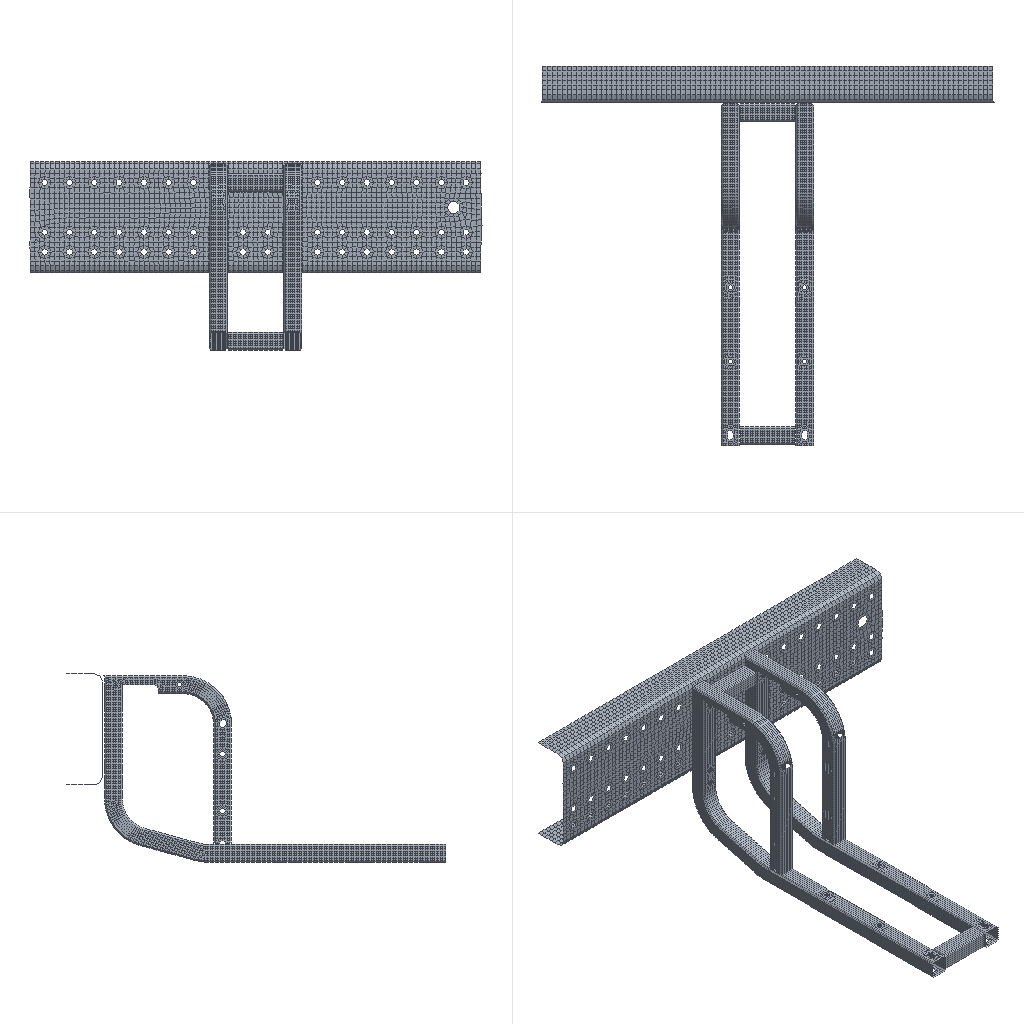Simulation study | nastran
Set-up summary:
category,name,step,type,value,unit,region
solver,nx_nastran
units,not stated in the deck,,not stated
analysis,deck,,static,static
analysis,solution,,SOL,101
load_step,SUBCASE 1,1,SUBCASE,SPC=6 LOAD=1
load_step,SUBCASE 2,2,SUBCASE,SPC=6 LOAD=2
load_step,SUBCASE 3,3,SUBCASE,SPC=6 LOAD=3
load_step,SUBCASE 4,4,SUBCASE,SPC=6 LOAD=4
load_step,requested,,,4
mesh,nodes,,,21323
mesh,elements,,,20706
element_type,CONM2,,mass,1
element_type,CQUAD4,,shell,20543
element_type,CTRIA3,,shell,162
load,load commands in deck,,count,4
bc,support commands in deck,,count,72
check,setup vs results,,match,"every grid point's frame and coordinates and every element id; grid points of CQUAD4, CTRIA3 elements"
Nastran input file, long lists of numbers shortened:
$$------------------------------------------------------------------------------$
$$                                                                              $
$$ NASTRAN Input Deck Generated by HyperMesh Version  : 9.0b121                 $
$$ Generated using HyperMesh-Nastran Template Version : 9.0b121
$$                                                                              $
$$   Template:  general                                                         $
$$                                                                              $
$$------------------------------------------------------------------------------$
$$------------------------------------------------------------------------------$
$$                      Executive Control Cards                                 $
$$------------------------------------------------------------------------------$
SOL 101
CEND
$$------------------------------------------------------------------------------$
$$                      Case Control Cards                                      $
$$------------------------------------------------------------------------------$
  DISPLACEMENT(PLOT) = ALL
  STRESS(PLOT) = ALL
  STRAIN(PLOT) = ALL
$
$HMNAME LOADSTEP               1"Step_X2g"
SUBCASE       1
  LABEL=        Step_X2g
  SPC =        6
  LOAD =        1
$
$HMNAME LOADSTEP               2"Step_Y2g"
SUBCASE       2
  LABEL=        Step_Y2g
  SPC =        6
  LOAD =        2
$
$HMNAME LOADSTEP               3"Step_Z2g"
SUBCASE       3
  LABEL=        Step_Z2g
  SPC =        6
  LOAD =        3
$
$HMNAME LOADSTEP               4"Step_Z-4g"
SUBCASE       4
  LABEL=        Step_Z-4g
  SPC =        6
  LOAD =        4
$$------------------------------------------------------------------------------$
$$                      Bulk Data Cards                                         $
$$------------------------------------------------------------------------------$
BEGIN BULK
PARAM,BAILOUT,-1
PARAM,POST,-1
$$
$$  GRID Data
$$
GRID          31        1732.005-658.5  -165.021
GRID          32        1732.005-661.979-165.021
$ (21321 more lines like these left out)
$$
$$  SPOINT Data
$$
$
$  CONM2 Elements
$
CONM2      18851  215425       00.02    0.0     0.0     0.0
$
$HMMOVE       11
$          18851
$
$$
$$------------------------------------------------------------------------------$
$$             Group Definitions                                                $
$$------------------------------------------------------------------------------$
$
$ RBE2 Elements - Single dependent node
$
RBE2      183220     317  123456  206486
RBE2      183221     316  123456  206487
$ (106 more lines like these left out)
$
$HMMOVE        9
$         183220THRU      183274   18129THRU       18138   18140THRU       18159
$          18161THRU       18170   18173THRU       18185
$
$$
$$ RBE2 Elements - Multiple dependent nodes
$$
RBE2       18850  215425  123456      32      33      34      35  203901+
+         203902  203903  203928  203929  203930  203931  203932  203933+
+         203934  204021     194  204022     252     253     273     274+
+            275     276     277     278     279     280     281     282+
+            283     284     287     288     289     290     291     292+
+            293     294     295     296     297     298     299     300+
+            301     302     303    6087  205562  205563  205564  205565+
+         205566  205567  205639  205640  205641  205642  205643  205644+
+         205645  205646  205647  205648  205649  205650  205651  205652+
+         205653  205654  205655  205656  205657  205658  205659  205660+
+         205661  205662    6890    6891    6892    6893    6894    7021+
+           7022    7023    7024  206018  206019  206020  206021  206022+
+         206023  206024  206025  207737  207738  207739  207740  207741+
+         207742  207743    9168  207767    9170    9171    9172    9173+
+           9174  207881  207882  207883  207897  207898  207918  207919+
+         207920  207921  207922  207923  207924  207925  207926  207927+
+         207928  207929  207930  207931  207932  207933  207934  207935+
+         207936  207937  207938  207939  207940  207941  207942  207943+
+         207944  207945  207946   14534   14535   14536   14537   14538+
+          14539  212201   14541  212231  212232  212233  212234  212235+
+         212236  212237   14739   14741   14742   14743   14744  212340+
+         212341   14747  212342  212343  212395  212396  212397  212398+
+         212399  212400  212714  212715  212716  212717  212718  212719+
+         212720  212723  212724  212741  212742  212743  212838  212839+
+         212840  212841  212842  215240  215241  215242  215243  215244+
+         215245  215246  215247  215256  215257  215258  215259  215260+
+         215261  215262  215280  215282  215283  215284  215285  215286+
+         215287  215288  215289  215290  215293  215294  215295  215296+
+         215297  215298   18671  215315  215316  215317  215318  215319+
+         215320  215321  215322  215323   18681   18682   18691   18692+
+         215324   18694   18695   18712  215334  215335   18715  215336+
+         215337  215338   18719  215347  215348   18740  215349  215350+
+         215351  215352   18791  215369  215370   18795  215371  215372+
+         215373  215374  215375   18801  215376  215377  215378  215379+
+         215380  215381   18843  215394  215395  215396  215397  215398+
+         215399  215400  215401  215402  215403  215404  215405  215406+
+         215407  215408  215409
RBE2      813136  846112  123456    3111    3112    3113    3114    3115+
+           3116    3117    3118    3119    3120    3121    3122    3123+
+           3124    3125    3126    3127    3128    3129    3130    3131+
+           3132    3133    3134    3696    3697    3698    3699    3700+
+           3701    3702    3703    3704    3705    3706    3707    3708+
+           3709    3710    3711    3712    3713    3714    3715    3716+
+           3717    3718    3719   71319   71320   71321   71322   71323+
+          71324   71325   71326   77189   77190   77191   77192   77193+
+          77194   77195   77196
RBE2      813137  846113  123456   71303   71304   71305   71306   71307+
+          71308   71309   71310   77165   77166   77167   77168   77169+
+          77170   77171   77172  209925  209926  209927  209928  209929+
+         209930  209931  209932  209933  209934  209935  209936  209937+
+         209938  209939  209940  209941  209942  209943  209944  209945+
+         209946  209947  209948  210396  210397  210398  210399  210400+
+         210401  210402  210403  210404  210405  210406  210407  210408+
+         210409  210410  210411  210412  210413  210414  210415  210416+
+         210417  210418  210419
RBE2      813138  846114  123456    3210    3211    3212    3213    3214+
+           3215    3216    3737    3738    3739    3740    3741    3742+
+           3743    3915    3916    3917    3918    3919    3920    3921+
+           3922    3923    3924    3925    3926    3927    3928    3929+
+           3930    3931    4122    4123    4124    4125    4126   69871+
+          69872   69873   69874   69875   69876   69877   69878   76481+
+          76482   76483   76484   76485   76486   76487   76488  207711+
+         207712  207713  207714  207715  207716  207717  207718
RBE2      813139  846115  123456   11897   11898   11899   11900   11901+
+          11902   11903   70623   70624   70625   70626   70627   70628+
+          70629   70630   76457   76458   76459   76460   76461   76462+
+          76463   76464  210437  210438  210439  210440  210441  210442+
+         210443  210615  210616  210617  210618  210619  210620  210621+
+         210622  210623  210624  210625  210626  210627  210628  210629+
+         210630  210631  210822  210823  210824  210825  210826  214675+
+         214676  214677  214678  214679  214680  214681  214682
$
$HMMOVE        9
$          18850  813136THRU      813139
$
$$
$$  CTRIA3 Data
$$
CTRIA3     69502       2   72070   72078   70294
CTRIA3     70999       2   69714   73125   73131
$ (160 more lines like these left out)
$
$HMMOVE  2801014
$          69502   70999  105895  107267  108257  108309
$
$ (28 more lines like these left out)
CQUAD4     69415       2   69010   69011   72029   72019
CQUAD4     69434       2   72019   72029   72041   72031
$ (20541 more lines like these left out)
$
$HMMOVE  2801014
$          69415   69434THRU       69435   69449   69452   69464   69468   69475
$          69483   69494THRU       69496   69510   69512THRU       69513   69517
$ (656 more lines like these left out)
PSHELL         2       16.0            1               1
$
$HMNAME PROP                   3"Pshell_400T" 4
$HWCOLOR PROP                  3       3
PSHELL         3       14.0            1               1
$$
$$------------------------------------------------------------------------------$
$$                      Material Definition Cards                               $
$$------------------------------------------------------------------------------$
$$--------------------------------------------------------------
$$ HYPERMESH TAGS
$$--------------------------------------------------------------
$$BEGIN TAGS
$$END TAGS
$$
$$  MAT1 Data
$
$HMNAME MAT                    1"Steel" "MAT1"
$HWCOLOR MAT                   1       3
MAT1           1210000.0        0.3     7.90E-09
$$
$$
$$
$$------------------------------------------------------------------------------$
$ (27 more lines like these left out)
GRAV           1        9800.0  2.0     0.0     0.0
$$
$HMNAME LOADCOL                2"Y2g"
$HWCOLOR LOADCOL               2       4
GRAV           2        9800.0  0.0     2.0     0.0
$$
$HMNAME LOADCOL                3"Z2g"
$HWCOLOR LOADCOL               3       5
GRAV           3        9800.0  0.0     0.0     2.0
$$
$HMNAME LOADCOL                4"Z-4g"
$HWCOLOR LOADCOL               4       6
GRAV           4        9800.0  0.0     0.0     -4.0
$$
$$
$$
$$
$$
$$
$$
$$
$$
$$
$$
$$  SPC Data
$$
SPC            6   79919  1234560.0
SPC            6   73165  1234560.0
SPC            6   73156  1234560.0
SPC            6   73177  1234560.0
$ (68 more lines like these left out)
$HMASSEM   28010       3 2801
$HMASSEM_IDS     2801014
$
ENDDATA
Results summary:
result,analysis,,,static
result,last_loadstep,,,4
result,primary field,,,displacements
result,max displacement,,,1.138,model units